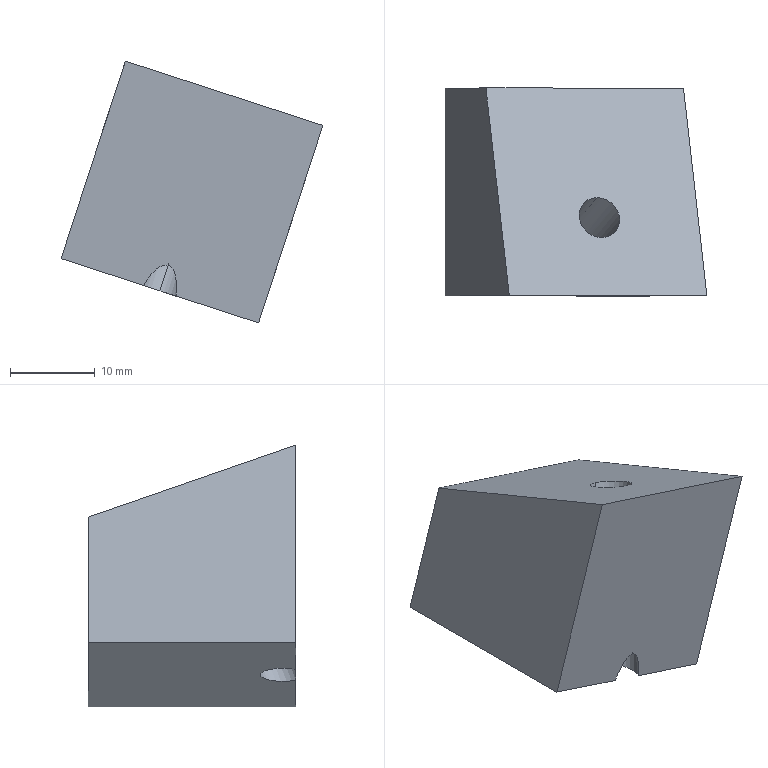Part | STEP file | 1 solid | 12 faces | box 30.872 x 24.5 x 30.872 mm | volume 11423 mm3 | plane 6 | cylinder 4 | cone 2 | commonest cylinder face diameters 4.165 x2 4.998 x2
STEP:
#1=CARTESIAN_POINT('',(0.,0.,0.));
#2=DIRECTION('',(0.,0.,1.));
#3=DIRECTION('',(1.,0.,0.));
#4=AXIS2_PLACEMENT_3D('',#1,#2,#3);
#5=CARTESIAN_POINT('',(844.273,-70.314,183.907));
#6=VERTEX_POINT('',#5);
#7=CARTESIAN_POINT('',(848.234,-70.314,182.62));
#8=VERTEX_POINT('',#7);
#9=CARTESIAN_POINT('',(846.254,-70.314,183.263));
#10=DIRECTION('',(0.,1.,0.));
#11=DIRECTION('',(-0.9511,0.,0.309));
#12=AXIS2_PLACEMENT_3D('',#9,#10,#11);
#13=CIRCLE('',#12,2.083);
#14=CARTESIAN_POINT('',(846.254,-70.314,183.263));
#15=DIRECTION('',(0.,1.,0.));
#16=DIRECTION('',(-0.9511,0.,0.309));
#17=AXIS2_PLACEMENT_3D('',#14,#15,#16);
#18=CONICAL_SURFACE('',#17,2.083,1.03);
#19=CARTESIAN_POINT('',(0.,0.));
#20=DIRECTION('',(1.,0.));
#21=VECTOR('',#20,1.);
#22=LINE('',#19,#21);
#23=(GEOMETRIC_REPRESENTATION_CONTEXT(2)PARAMETRIC_REPRESENTATION_CONTEXT()REPRESENTATION_CONTEXT('',''));
#24=DEFINITIONAL_REPRESENTATION('',(#22),#23);
#25=PCURVE('',#18,#24);
#26=CARTESIAN_POINT('',(846.254,-58.309,183.263));
#27=DIRECTION('',(0.,1.,0.));
#28=DIRECTION('',(-0.9511,0.,0.309));
#29=AXIS2_PLACEMENT_3D('',#26,#27,#28);
#30=CYLINDRICAL_SURFACE('',#29,2.083);
#31=CARTESIAN_POINT('',(0.,-12.005));
#32=DIRECTION('',(1.,0.));
#33=VECTOR('',#32,1.);
#34=LINE('',#31,#33);
#35=(GEOMETRIC_REPRESENTATION_CONTEXT(2)PARAMETRIC_REPRESENTATION_CONTEXT()REPRESENTATION_CONTEXT('',''));
#36=DEFINITIONAL_REPRESENTATION('',(#34),#35);
#37=PCURVE('',#30,#36);
#38=SURFACE_CURVE('',#13,(#25,#37),.PCURVE_S1.);
#39=EDGE_CURVE('',#6,#8,#38,.T.);
#40=ORIENTED_EDGE('',*,*,#39,.F.);
#41=CARTESIAN_POINT('',(846.254,-71.565,183.263));
#42=VERTEX_POINT('',#41);
#43=CARTESIAN_POINT('',(844.273,-70.314,183.907));
#44=DIRECTION('',(-0.8152,0.515,0.2649));
#45=VECTOR('',#44,1.);
#46=LINE('',#43,#45);
#47=CARTESIAN_POINT('',(0.,-1.251));
#48=CARTESIAN_POINT('',(0.,-1.232));
#49=CARTESIAN_POINT('',(0.,-1.194));
#50=CARTESIAN_POINT('',(0.,-1.138));
#51=CARTESIAN_POINT('',(0.,-1.081));
#52=CARTESIAN_POINT('',(0.,-1.024));
#53=CARTESIAN_POINT('',(0.,-0.9669));
#54=CARTESIAN_POINT('',(0.,-0.91));
#55=CARTESIAN_POINT('',(0.,-0.8532));
#56=CARTESIAN_POINT('',(0.,-0.7963));
#57=CARTESIAN_POINT('',(0.,-0.7394));
#58=CARTESIAN_POINT('',(0.,-0.6825));
#59=CARTESIAN_POINT('',(0.,-0.6256));
#60=CARTESIAN_POINT('',(0.,-0.5688));
#61=CARTESIAN_POINT('',(0.,-0.5119));
#62=CARTESIAN_POINT('',(0.,-0.455));
#63=CARTESIAN_POINT('',(0.,-0.3981));
#64=CARTESIAN_POINT('',(0.,-0.3413));
#65=CARTESIAN_POINT('',(0.,-0.2844));
#66=CARTESIAN_POINT('',(0.,-0.2275));
#67=CARTESIAN_POINT('',(0.,-0.1706));
#68=CARTESIAN_POINT('',(0.,-0.1138));
#69=CARTESIAN_POINT('',(0.,-0.05688));
#70=CARTESIAN_POINT('',(0.,-0.01896));
#71=CARTESIAN_POINT('',(0.,0.));
#72=B_SPLINE_CURVE_WITH_KNOTS('',3,(#47,#48,#49,#50,#51,#52,#53,#54,#55,#56,#57,#58,#59,#60,#61,#62,#63,#64,#65,#66,#67,#68,#69,#70,#71),.UNSPECIFIED.,.F.,.F.,(4,1,1,1,1,1,1,1,1,1,1,1,1,1,1,1,1,1,1,1,1,1,4),(-2.43,-2.319,-2.209,-2.098,-1.988,-1.877,-1.767,-1.656,-1.546,-1.436,-1.325,-1.215,-1.104,-0.9939,-0.8835,-0.773,-0.6626,-0.5522,-0.4417,-0.3313,-0.2209,-0.1104,0.),.UNSPECIFIED.);
#73=(GEOMETRIC_REPRESENTATION_CONTEXT(2)PARAMETRIC_REPRESENTATION_CONTEXT()REPRESENTATION_CONTEXT('',''));
#74=DEFINITIONAL_REPRESENTATION('',(#72),#73);
#75=PCURVE('',#18,#74);
#76=CARTESIAN_POINT('',(846.254,-70.314,183.263));
#77=DIRECTION('',(0.,1.,0.));
#78=DIRECTION('',(-0.9511,0.,0.309));
#79=AXIS2_PLACEMENT_3D('',#76,#77,#78);
#80=CONICAL_SURFACE('',#79,2.083,1.03);
#81=CARTESIAN_POINT('',(6.283,-1.251));
#82=CARTESIAN_POINT('',(6.283,-1.232));
#83=CARTESIAN_POINT('',(6.283,-1.194));
#84=CARTESIAN_POINT('',(6.283,-1.138));
#85=CARTESIAN_POINT('',(6.283,-1.081));
#86=CARTESIAN_POINT('',(6.283,-1.024));
#87=CARTESIAN_POINT('',(6.283,-0.9669));
#88=CARTESIAN_POINT('',(6.283,-0.91));
#89=CARTESIAN_POINT('',(6.283,-0.8532));
#90=CARTESIAN_POINT('',(6.283,-0.7963));
#91=CARTESIAN_POINT('',(6.283,-0.7394));
#92=CARTESIAN_POINT('',(6.283,-0.6825));
#93=CARTESIAN_POINT('',(6.283,-0.6256));
#94=CARTESIAN_POINT('',(6.283,-0.5688));
#95=CARTESIAN_POINT('',(6.283,-0.5119));
#96=CARTESIAN_POINT('',(6.283,-0.455));
#97=CARTESIAN_POINT('',(6.283,-0.3981));
#98=CARTESIAN_POINT('',(6.283,-0.3413));
#99=CARTESIAN_POINT('',(6.283,-0.2844));
#100=CARTESIAN_POINT('',(6.283,-0.2275));
#101=CARTESIAN_POINT('',(6.283,-0.1706));
#102=CARTESIAN_POINT('',(6.283,-0.1138));
#103=CARTESIAN_POINT('',(6.283,-0.05688));
#104=CARTESIAN_POINT('',(6.283,-0.01896));
#105=CARTESIAN_POINT('',(6.283,0.));
#106=B_SPLINE_CURVE_WITH_KNOTS('',3,(#81,#82,#83,#84,#85,#86,#87,#88,#89,#90,#91,#92,#93,#94,#95,#96,#97,#98,#99,#100,#101,#102,#103,#104,#105),.UNSPECIFIED.,.F.,.F.,(4,1,1,1,1,1,1,1,1,1,1,1,1,1,1,1,1,1,1,1,1,1,4),(-2.43,-2.319,-2.209,-2.098,-1.988,-1.877,-1.767,-1.656,-1.546,-1.436,-1.325,-1.215,-1.104,-0.9939,-0.8835,-0.773,-0.6626,-0.5522,-0.4417,-0.3313,-0.2209,-0.1104,0.),.UNSPECIFIED.);
#107=(GEOMETRIC_REPRESENTATION_CONTEXT(2)PARAMETRIC_REPRESENTATION_CONTEXT()REPRESENTATION_CONTEXT('',''));
#108=DEFINITIONAL_REPRESENTATION('',(#106),#107);
#109=PCURVE('',#80,#108);
#110=SURFACE_CURVE('',#46,(#75,#109),.PCURVE_S1.);
#111=EDGE_CURVE('',#42,#6,#110,.T.);
#112=ORIENTED_EDGE('',*,*,#111,.F.);
#113=CARTESIAN_POINT('',(848.234,-70.314,182.62));
#114=DIRECTION('',(0.8152,0.515,-0.2649));
#115=VECTOR('',#114,1.);
#116=LINE('',#113,#115);
#117=CARTESIAN_POINT('',(3.142,-1.251));
#118=CARTESIAN_POINT('',(3.142,-1.232));
#119=CARTESIAN_POINT('',(3.142,-1.194));
#120=CARTESIAN_POINT('',(3.142,-1.138));
#121=CARTESIAN_POINT('',(3.142,-1.081));
#122=CARTESIAN_POINT('',(3.142,-1.024));
#123=CARTESIAN_POINT('',(3.142,-0.9669));
#124=CARTESIAN_POINT('',(3.142,-0.91));
#125=CARTESIAN_POINT('',(3.142,-0.8532));
#126=CARTESIAN_POINT('',(3.142,-0.7963));
#127=CARTESIAN_POINT('',(3.142,-0.7394));
#128=CARTESIAN_POINT('',(3.142,-0.6825));
#129=CARTESIAN_POINT('',(3.142,-0.6256));
#130=CARTESIAN_POINT('',(3.142,-0.5688));
#131=CARTESIAN_POINT('',(3.142,-0.5119));
#132=CARTESIAN_POINT('',(3.142,-0.455));
#133=CARTESIAN_POINT('',(3.142,-0.3981));
#134=CARTESIAN_POINT('',(3.142,-0.3413));
#135=CARTESIAN_POINT('',(3.142,-0.2844));
#136=CARTESIAN_POINT('',(3.142,-0.2275));
#137=CARTESIAN_POINT('',(3.142,-0.1706));
#138=CARTESIAN_POINT('',(3.142,-0.1138));
#139=CARTESIAN_POINT('',(3.142,-0.05688));
#140=CARTESIAN_POINT('',(3.142,-0.01896));
#141=CARTESIAN_POINT('',(3.142,0.));
#142=B_SPLINE_CURVE_WITH_KNOTS('',3,(#117,#118,#119,#120,#121,#122,#123,#124,#125,#126,#127,#128,#129,#130,#131,#132,#133,#134,#135,#136,#137,#138,#139,#140,#141),.UNSPECIFIED.,.F.,.F.,(4,1,1,1,1,1,1,1,1,1,1,1,1,1,1,1,1,1,1,1,1,1,4),(-2.43,-2.319,-2.209,-2.098,-1.988,-1.877,-1.767,-1.656,-1.546,-1.436,-1.325,-1.215,-1.104,-0.9939,-0.8835,-0.773,-0.6626,-0.5522,-0.4417,-0.3313,-0.2209,-0.1104,0.),.UNSPECIFIED.);
#143=(GEOMETRIC_REPRESENTATION_CONTEXT(2)PARAMETRIC_REPRESENTATION_CONTEXT()REPRESENTATION_CONTEXT('',''));
#144=DEFINITIONAL_REPRESENTATION('',(#142),#143);
#145=PCURVE('',#18,#144);
#146=CARTESIAN_POINT('',(3.142,-1.251));
#147=CARTESIAN_POINT('',(3.142,-1.232));
#148=CARTESIAN_POINT('',(3.142,-1.194));
#149=CARTESIAN_POINT('',(3.142,-1.138));
#150=CARTESIAN_POINT('',(3.142,-1.081));
#151=CARTESIAN_POINT('',(3.142,-1.024));
#152=CARTESIAN_POINT('',(3.142,-0.9669));
#153=CARTESIAN_POINT('',(3.142,-0.91));
#154=CARTESIAN_POINT('',(3.142,-0.8532));
#155=CARTESIAN_POINT('',(3.142,-0.7963));
#156=CARTESIAN_POINT('',(3.142,-0.7394));
#157=CARTESIAN_POINT('',(3.142,-0.6825));
#158=CARTESIAN_POINT('',(3.142,-0.6256));
#159=CARTESIAN_POINT('',(3.142,-0.5688));
#160=CARTESIAN_POINT('',(3.142,-0.5119));
#161=CARTESIAN_POINT('',(3.142,-0.455));
#162=CARTESIAN_POINT('',(3.142,-0.3981));
#163=CARTESIAN_POINT('',(3.142,-0.3413));
#164=CARTESIAN_POINT('',(3.142,-0.2844));
#165=CARTESIAN_POINT('',(3.142,-0.2275));
#166=CARTESIAN_POINT('',(3.142,-0.1706));
#167=CARTESIAN_POINT('',(3.142,-0.1138));
#168=CARTESIAN_POINT('',(3.142,-0.05688));
#169=CARTESIAN_POINT('',(3.142,-0.01896));
#170=CARTESIAN_POINT('',(3.142,0.));
#171=B_SPLINE_CURVE_WITH_KNOTS('',3,(#146,#147,#148,#149,#150,#151,#152,#153,#154,#155,#156,#157,#158,#159,#160,#161,#162,#163,#164,#165,#166,#167,#168,#169,#170),.UNSPECIFIED.,.F.,.F.,(4,1,1,1,1,1,1,1,1,1,1,1,1,1,1,1,1,1,1,1,1,1,4),(-2.43,-2.319,-2.209,-2.098,-1.988,-1.877,-1.767,-1.656,-1.546,-1.436,-1.325,-1.215,-1.104,-0.9939,-0.8835,-0.773,-0.6626,-0.5522,-0.4417,-0.3313,-0.2209,-0.1104,0.),.UNSPECIFIED.);
#172=(GEOMETRIC_REPRESENTATION_CONTEXT(2)PARAMETRIC_REPRESENTATION_CONTEXT()REPRESENTATION_CONTEXT('',''));
#173=DEFINITIONAL_REPRESENTATION('',(#171),#172);
#174=PCURVE('',#80,#173);
#175=SURFACE_CURVE('',#116,(#145,#174),.PCURVE_S1.);
#176=EDGE_CURVE('',#42,#8,#175,.T.);
#177=ORIENTED_EDGE('',*,*,#176,.T.);
#178=EDGE_LOOP('',(#40,#112,#177));
#179=FACE_BOUND('',#178,.F.);
#180=ADVANCED_FACE('',(#179),#18,.F.);
#181=CARTESIAN_POINT('',(844.273,-58.309,183.907));
#182=VERTEX_POINT('',#181);
#183=CARTESIAN_POINT('',(848.234,-58.309,182.62));
#184=VERTEX_POINT('',#183);
#185=CARTESIAN_POINT('',(846.254,-58.309,183.263));
#186=DIRECTION('',(0.,1.,0.));
#187=DIRECTION('',(-0.9511,0.,0.309));
#188=AXIS2_PLACEMENT_3D('',#185,#186,#187);
#189=CIRCLE('',#188,2.083);
#190=CARTESIAN_POINT('',(0.,0.));
#191=DIRECTION('',(1.,0.));
#192=VECTOR('',#191,1.);
#193=LINE('',#190,#192);
#194=(GEOMETRIC_REPRESENTATION_CONTEXT(2)PARAMETRIC_REPRESENTATION_CONTEXT()REPRESENTATION_CONTEXT('',''));
#195=DEFINITIONAL_REPRESENTATION('',(#193),#194);
#196=PCURVE('',#30,#195);
#197=CARTESIAN_POINT('',(837.147,-58.309,194.878));
#198=DIRECTION('',(0.,-1.,0.));
#199=DIRECTION('',(0.9511,0.,-0.309));
#200=AXIS2_PLACEMENT_3D('',#197,#198,#199);
#201=PLANE('',#200);
#202=CARTESIAN_POINT('',(10.168,-8.233));
#203=CARTESIAN_POINT('',(10.168,-4.626));
#204=CARTESIAN_POINT('',(13.291,-6.429));
#205=CARTESIAN_POINT('',(16.415,-8.233));
#206=CARTESIAN_POINT('',(13.291,-10.036));
#207=CARTESIAN_POINT('',(10.168,-11.84));
#208=CARTESIAN_POINT('',(10.168,-8.233));
#209=(BOUNDED_CURVE()B_SPLINE_CURVE(2,(#202,#203,#204,#205,#206,#207,#208),.UNSPECIFIED.,.T.,.F.)B_SPLINE_CURVE_WITH_KNOTS((1,2,2,2,2,1),(-2.094,0.,2.094,4.189,6.283,8.378),.UNSPECIFIED.)CURVE()GEOMETRIC_REPRESENTATION_ITEM()RATIONAL_B_SPLINE_CURVE((1.,0.5,1.,0.5,1.,0.5,1.))REPRESENTATION_ITEM(''));
#210=(GEOMETRIC_REPRESENTATION_CONTEXT(2)PARAMETRIC_REPRESENTATION_CONTEXT()REPRESENTATION_CONTEXT('',''));
#211=DEFINITIONAL_REPRESENTATION('',(#209),#210);
#212=PCURVE('',#201,#211);
#213=SURFACE_CURVE('',#189,(#196,#212),.PCURVE_S1.);
#214=EDGE_CURVE('',#182,#184,#213,.T.);
#215=ORIENTED_EDGE('',*,*,#214,.F.);
#216=CARTESIAN_POINT('',(844.273,-58.309,183.907));
#217=DIRECTION('',(0.,1.,0.));
#218=VECTOR('',#217,1.);
#219=LINE('',#216,#218);
#220=CARTESIAN_POINT('',(0.,0.));
#221=DIRECTION('',(0.,1.));
#222=VECTOR('',#221,1.);
#223=LINE('',#220,#222);
#224=(GEOMETRIC_REPRESENTATION_CONTEXT(2)PARAMETRIC_REPRESENTATION_CONTEXT()REPRESENTATION_CONTEXT('',''));
#225=DEFINITIONAL_REPRESENTATION('',(#223),#224);
#226=PCURVE('',#30,#225);
#227=CARTESIAN_POINT('',(846.254,-58.309,183.263));
#228=DIRECTION('',(0.,1.,0.));
#229=DIRECTION('',(-0.9511,0.,0.309));
#230=AXIS2_PLACEMENT_3D('',#227,#228,#229);
#231=CYLINDRICAL_SURFACE('',#230,2.083);
#232=CARTESIAN_POINT('',(6.283,0.));
#233=DIRECTION('',(0.,1.));
#234=VECTOR('',#233,1.);
#235=LINE('',#232,#234);
#236=(GEOMETRIC_REPRESENTATION_CONTEXT(2)PARAMETRIC_REPRESENTATION_CONTEXT()REPRESENTATION_CONTEXT('',''));
#237=DEFINITIONAL_REPRESENTATION('',(#235),#236);
#238=PCURVE('',#231,#237);
#239=SURFACE_CURVE('',#219,(#226,#238),.PCURVE_S1.);
#240=EDGE_CURVE('',#6,#182,#239,.T.);
#241=ORIENTED_EDGE('',*,*,#240,.F.);
#242=ORIENTED_EDGE('',*,*,#39,.T.);
#243=CARTESIAN_POINT('',(848.234,-58.309,182.62));
#244=DIRECTION('',(0.,1.,0.));
#245=VECTOR('',#244,1.);
#246=LINE('',#243,#245);
#247=CARTESIAN_POINT('',(3.142,0.));
#248=DIRECTION('',(0.,1.));
#249=VECTOR('',#248,1.);
#250=LINE('',#247,#249);
#251=(GEOMETRIC_REPRESENTATION_CONTEXT(2)PARAMETRIC_REPRESENTATION_CONTEXT()REPRESENTATION_CONTEXT('',''));
#252=DEFINITIONAL_REPRESENTATION('',(#250),#251);
#253=PCURVE('',#30,#252);
#254=CARTESIAN_POINT('',(3.142,0.));
#255=DIRECTION('',(0.,1.));
#256=VECTOR('',#255,1.);
#257=LINE('',#254,#256);
#258=(GEOMETRIC_REPRESENTATION_CONTEXT(2)PARAMETRIC_REPRESENTATION_CONTEXT()REPRESENTATION_CONTEXT('',''));
#259=DEFINITIONAL_REPRESENTATION('',(#257),#258);
#260=PCURVE('',#231,#259);
#261=SURFACE_CURVE('',#246,(#253,#260),.PCURVE_S1.);
#262=EDGE_CURVE('',#8,#184,#261,.T.);
#263=ORIENTED_EDGE('',*,*,#262,.T.);
#264=EDGE_LOOP('',(#215,#241,#242,#263));
#265=FACE_BOUND('',#264,.F.);
#266=ADVANCED_FACE('',(#265),#30,.F.);
#267=CARTESIAN_POINT('',(855.633,-82.809,172.487));
#268=VERTEX_POINT('',#267);
#269=CARTESIAN_POINT('',(845.938,-82.809,175.638));
#270=VERTEX_POINT('',#269);
#271=CARTESIAN_POINT('',(832.332,-82.809,180.058));
#272=DIRECTION('',(-0.9511,0.,0.309));
#273=VECTOR('',#272,1.);
#274=LINE('',#271,#273);
#275=CARTESIAN_POINT('',(832.332,-58.309,180.058));
#276=DIRECTION('',(0.309,0.,0.9511));
#277=DIRECTION('',(0.,1.,0.));
#278=AXIS2_PLACEMENT_3D('',#275,#276,#277);
#279=PLANE('',#278);
#280=CARTESIAN_POINT('',(-24.5,0.));
#281=DIRECTION('',(0.,1.));
#282=VECTOR('',#281,1.);
#283=LINE('',#280,#282);
#284=(GEOMETRIC_REPRESENTATION_CONTEXT(2)PARAMETRIC_REPRESENTATION_CONTEXT()REPRESENTATION_CONTEXT('',''));
#285=DEFINITIONAL_REPRESENTATION('',(#283),#284);
#286=PCURVE('',#279,#285);
#287=CARTESIAN_POINT('',(832.332,-82.809,180.058));
#288=DIRECTION('',(0.,1.,0.));
#289=DIRECTION('',(0.309,0.,0.9511));
#290=AXIS2_PLACEMENT_3D('',#287,#288,#289);
#291=PLANE('',#290);
#292=CARTESIAN_POINT('',(0.,0.));
#293=DIRECTION('',(0.,-1.));
#294=VECTOR('',#293,1.);
#295=LINE('',#292,#294);
#296=(GEOMETRIC_REPRESENTATION_CONTEXT(2)PARAMETRIC_REPRESENTATION_CONTEXT()REPRESENTATION_CONTEXT('',''));
#297=DEFINITIONAL_REPRESENTATION('',(#295),#296);
#298=PCURVE('',#291,#297);
#299=SURFACE_CURVE('',#274,(#286,#298),.PCURVE_S1.);
#300=EDGE_CURVE('',#268,#270,#299,.T.);
#301=ORIENTED_EDGE('',*,*,#300,.T.);
#302=CARTESIAN_POINT('',(843.983,-78.638,176.273));
#303=VERTEX_POINT('',#302);
#304=CARTESIAN_POINT('',(845.938,-82.809,175.638));
#305=CARTESIAN_POINT('',(847.178,-80.8,175.235));
#306=CARTESIAN_POINT('',(846.165,-78.638,175.564));
#307=CARTESIAN_POINT('',(843.983,-78.638,176.273));
#308=(BOUNDED_CURVE()B_SPLINE_CURVE(3,(#304,#305,#306,#307),.UNSPECIFIED.,.F.,.F.)B_SPLINE_CURVE_WITH_KNOTS((4,4),(4.108,6.283),.PIECEWISE_BEZIER_KNOTS.)CURVE()GEOMETRIC_REPRESENTATION_ITEM()RATIONAL_B_SPLINE_CURVE((1.,0.643,0.643,1.))REPRESENTATION_ITEM(''));
#309=CARTESIAN_POINT('',(-24.5,-14.306));
#310=CARTESIAN_POINT('',(-22.491,-15.61));
#311=CARTESIAN_POINT('',(-20.329,-14.544));
#312=CARTESIAN_POINT('',(-20.329,-12.25));
#313=(BOUNDED_CURVE()B_SPLINE_CURVE(3,(#309,#310,#311,#312),.UNSPECIFIED.,.F.,.F.)B_SPLINE_CURVE_WITH_KNOTS((4,4),(4.108,6.283),.PIECEWISE_BEZIER_KNOTS.)CURVE()GEOMETRIC_REPRESENTATION_ITEM()RATIONAL_B_SPLINE_CURVE((1.,0.643,0.643,1.))REPRESENTATION_ITEM(''));
#314=(GEOMETRIC_REPRESENTATION_CONTEXT(2)PARAMETRIC_REPRESENTATION_CONTEXT()REPRESENTATION_CONTEXT('',''));
#315=DEFINITIONAL_REPRESENTATION('',(#313),#314);
#316=PCURVE('',#279,#315);
#317=CARTESIAN_POINT('',(850.518,-73.6,196.386));
#318=DIRECTION('',(0.2904,0.342,0.8937));
#319=DIRECTION('',(-0.1057,0.9397,-0.3253));
#320=AXIS2_PLACEMENT_3D('',#317,#318,#319);
#321=CYLINDRICAL_SURFACE('',#320,2.499);
#322=CARTESIAN_POINT('',(4.108,-23.022));
#323=CARTESIAN_POINT('',(4.135,-23.002));
#324=CARTESIAN_POINT('',(4.19,-22.96));
#325=CARTESIAN_POINT('',(4.276,-22.89));
#326=CARTESIAN_POINT('',(4.366,-22.814));
#327=CARTESIAN_POINT('',(4.46,-22.733));
#328=CARTESIAN_POINT('',(4.558,-22.646));
#329=CARTESIAN_POINT('',(4.659,-22.554));
#330=CARTESIAN_POINT('',(4.762,-22.46));
#331=CARTESIAN_POINT('',(4.868,-22.364));
#332=CARTESIAN_POINT('',(4.976,-22.268));
#333=CARTESIAN_POINT('',(5.086,-22.173));
#334=CARTESIAN_POINT('',(5.195,-22.082));
#335=CARTESIAN_POINT('',(5.305,-21.996));
#336=CARTESIAN_POINT('',(5.415,-21.917));
#337=CARTESIAN_POINT('',(5.523,-21.845));
#338=CARTESIAN_POINT('',(5.629,-21.782));
#339=CARTESIAN_POINT('',(5.732,-21.729));
#340=CARTESIAN_POINT('',(5.833,-21.685));
#341=CARTESIAN_POINT('',(5.931,-21.65));
#342=CARTESIAN_POINT('',(6.025,-21.625));
#343=CARTESIAN_POINT('',(6.115,-21.608));
#344=CARTESIAN_POINT('',(6.201,-21.598));
#345=CARTESIAN_POINT('',(6.256,-21.596));
#346=CARTESIAN_POINT('',(6.283,-21.596));
#347=B_SPLINE_CURVE_WITH_KNOTS('',3,(#322,#323,#324,#325,#326,#327,#328,#329,#330,#331,#332,#333,#334,#335,#336,#337,#338,#339,#340,#341,#342,#343,#344,#345,#346),.UNSPECIFIED.,.F.,.F.,(4,1,1,1,1,1,1,1,1,1,1,1,1,1,1,1,1,1,1,1,1,1,4),(4.108,4.207,4.306,4.404,4.503,4.602,4.701,4.8,4.899,4.998,5.097,5.195,5.294,5.393,5.492,5.591,5.69,5.789,5.888,5.987,6.085,6.184,6.283),.QUASI_UNIFORM_KNOTS.);
#348=(GEOMETRIC_REPRESENTATION_CONTEXT(2)PARAMETRIC_REPRESENTATION_CONTEXT()REPRESENTATION_CONTEXT('',''));
#349=DEFINITIONAL_REPRESENTATION('',(#347),#348);
#350=PCURVE('',#321,#349);
#351=SURFACE_CURVE('',#308,(#316,#350),.PCURVE_S1.);
#352=EDGE_CURVE('',#270,#303,#351,.T.);
#353=ORIENTED_EDGE('',*,*,#352,.T.);
#354=CARTESIAN_POINT('',(842.027,-82.809,176.908));
#355=VERTEX_POINT('',#354);
#356=CARTESIAN_POINT('',(843.983,-78.638,176.273));
#357=CARTESIAN_POINT('',(841.8,-78.638,176.982));
#358=CARTESIAN_POINT('',(840.787,-80.8,177.311));
#359=CARTESIAN_POINT('',(842.027,-82.809,176.908));
#360=(BOUNDED_CURVE()B_SPLINE_CURVE(3,(#356,#357,#358,#359),.UNSPECIFIED.,.F.,.F.)B_SPLINE_CURVE_WITH_KNOTS((4,4),(0.,2.175),.PIECEWISE_BEZIER_KNOTS.)CURVE()GEOMETRIC_REPRESENTATION_ITEM()RATIONAL_B_SPLINE_CURVE((1.,0.643,0.643,1.))REPRESENTATION_ITEM(''));
#361=CARTESIAN_POINT('',(-20.329,-12.25));
#362=CARTESIAN_POINT('',(-20.329,-9.956));
#363=CARTESIAN_POINT('',(-22.491,-8.89));
#364=CARTESIAN_POINT('',(-24.5,-10.194));
#365=(BOUNDED_CURVE()B_SPLINE_CURVE(3,(#361,#362,#363,#364),.UNSPECIFIED.,.F.,.F.)B_SPLINE_CURVE_WITH_KNOTS((4,4),(0.,2.175),.PIECEWISE_BEZIER_KNOTS.)CURVE()GEOMETRIC_REPRESENTATION_ITEM()RATIONAL_B_SPLINE_CURVE((1.,0.643,0.643,1.))REPRESENTATION_ITEM(''));
#366=(GEOMETRIC_REPRESENTATION_CONTEXT(2)PARAMETRIC_REPRESENTATION_CONTEXT()REPRESENTATION_CONTEXT('',''));
#367=DEFINITIONAL_REPRESENTATION('',(#365),#366);
#368=PCURVE('',#279,#367);
#369=CARTESIAN_POINT('',(850.518,-73.6,196.386));
#370=DIRECTION('',(0.2904,0.342,0.8937));
#371=DIRECTION('',(-0.1057,0.9397,-0.3253));
#372=AXIS2_PLACEMENT_3D('',#369,#370,#371);
#373=CYLINDRICAL_SURFACE('',#372,2.499);
#374=CARTESIAN_POINT('',(0.,-21.596));
#375=CARTESIAN_POINT('',(0.02683,-21.596));
#376=CARTESIAN_POINT('',(0.08182,-21.598));
#377=CARTESIAN_POINT('',(0.1682,-21.608));
#378=CARTESIAN_POINT('',(0.2585,-21.625));
#379=CARTESIAN_POINT('',(0.3525,-21.65));
#380=CARTESIAN_POINT('',(0.45,-21.685));
#381=CARTESIAN_POINT('',(0.5508,-21.729));
#382=CARTESIAN_POINT('',(0.6544,-21.782));
#383=CARTESIAN_POINT('',(0.7605,-21.845));
#384=CARTESIAN_POINT('',(0.8685,-21.917));
#385=CARTESIAN_POINT('',(0.9778,-21.996));
#386=CARTESIAN_POINT('',(1.088,-22.082));
#387=CARTESIAN_POINT('',(1.198,-22.173));
#388=CARTESIAN_POINT('',(1.307,-22.268));
#389=CARTESIAN_POINT('',(1.415,-22.364));
#390=CARTESIAN_POINT('',(1.521,-22.46));
#391=CARTESIAN_POINT('',(1.625,-22.554));
#392=CARTESIAN_POINT('',(1.725,-22.646));
#393=CARTESIAN_POINT('',(1.823,-22.733));
#394=CARTESIAN_POINT('',(1.917,-22.814));
#395=CARTESIAN_POINT('',(2.007,-22.89));
#396=CARTESIAN_POINT('',(2.094,-22.96));
#397=CARTESIAN_POINT('',(2.149,-23.002));
#398=CARTESIAN_POINT('',(2.175,-23.022));
#399=B_SPLINE_CURVE_WITH_KNOTS('',3,(#374,#375,#376,#377,#378,#379,#380,#381,#382,#383,#384,#385,#386,#387,#388,#389,#390,#391,#392,#393,#394,#395,#396,#397,#398),.UNSPECIFIED.,.F.,.F.,(4,1,1,1,1,1,1,1,1,1,1,1,1,1,1,1,1,1,1,1,1,1,4),(0.,0.09888,0.1978,0.2966,0.3955,0.4944,0.5933,0.6922,0.7911,0.8899,0.9888,1.088,1.187,1.285,1.384,1.483,1.582,1.681,1.78,1.879,1.978,2.077,2.175),.QUASI_UNIFORM_KNOTS.);
#400=(GEOMETRIC_REPRESENTATION_CONTEXT(2)PARAMETRIC_REPRESENTATION_CONTEXT()REPRESENTATION_CONTEXT('',''));
#401=DEFINITIONAL_REPRESENTATION('',(#399),#400);
#402=PCURVE('',#373,#401);
#403=SURFACE_CURVE('',#360,(#368,#402),.PCURVE_S1.);
#404=EDGE_CURVE('',#303,#355,#403,.T.);
#405=ORIENTED_EDGE('',*,*,#404,.T.);
#406=CARTESIAN_POINT('',(832.332,-82.809,180.058));
#407=VERTEX_POINT('',#406);
#408=CARTESIAN_POINT('',(832.332,-82.809,180.058));
#409=DIRECTION('',(-0.9511,0.,0.309));
#410=VECTOR('',#409,1.);
#411=LINE('',#408,#410);
#412=CARTESIAN_POINT('',(-24.5,0.));
#413=DIRECTION('',(0.,1.));
#414=VECTOR('',#413,1.);
#415=LINE('',#412,#414);
#416=(GEOMETRIC_REPRESENTATION_CONTEXT(2)PARAMETRIC_REPRESENTATION_CONTEXT()REPRESENTATION_CONTEXT('',''));
#417=DEFINITIONAL_REPRESENTATION('',(#415),#416);
#418=PCURVE('',#279,#417);
#419=CARTESIAN_POINT('',(0.,0.));
#420=DIRECTION('',(0.,-1.));
#421=VECTOR('',#420,1.);
#422=LINE('',#419,#421);
#423=(GEOMETRIC_REPRESENTATION_CONTEXT(2)PARAMETRIC_REPRESENTATION_CONTEXT()REPRESENTATION_CONTEXT('',''));
#424=DEFINITIONAL_REPRESENTATION('',(#422),#423);
#425=PCURVE('',#291,#424);
#426=SURFACE_CURVE('',#411,(#418,#425),.PCURVE_S1.);
#427=EDGE_CURVE('',#355,#407,#426,.T.);
#428=ORIENTED_EDGE('',*,*,#427,.T.);
#429=CARTESIAN_POINT('',(832.332,-58.309,180.058));
#430=VERTEX_POINT('',#429);
#431=CARTESIAN_POINT('',(832.332,-82.809,180.058));
#432=DIRECTION('',(0.,-1.,0.));
#433=VECTOR('',#432,1.);
#434=LINE('',#431,#433);
#435=CARTESIAN_POINT('',(-24.5,0.));
#436=DIRECTION('',(-1.,0.));
#437=VECTOR('',#436,1.);
#438=LINE('',#435,#437);
#439=(GEOMETRIC_REPRESENTATION_CONTEXT(2)PARAMETRIC_REPRESENTATION_CONTEXT()REPRESENTATION_CONTEXT('',''));
#440=DEFINITIONAL_REPRESENTATION('',(#438),#439);
#441=PCURVE('',#279,#440);
#442=CARTESIAN_POINT('',(832.332,-82.809,180.058));
#443=DIRECTION('',(-0.9511,0.,0.309));
#444=DIRECTION('',(0.309,0.,0.9511));
#445=AXIS2_PLACEMENT_3D('',#442,#443,#444);
#446=PLANE('',#445);
#447=CARTESIAN_POINT('',(0.,0.));
#448=DIRECTION('',(0.,-1.));
#449=VECTOR('',#448,1.);
#450=LINE('',#447,#449);
#451=(GEOMETRIC_REPRESENTATION_CONTEXT(2)PARAMETRIC_REPRESENTATION_CONTEXT()REPRESENTATION_CONTEXT('',''));
#452=DEFINITIONAL_REPRESENTATION('',(#450),#451);
#453=PCURVE('',#446,#452);
#454=SURFACE_CURVE('',#434,(#441,#453),.PCURVE_S1.);
#455=EDGE_CURVE('',#430,#407,#454,.T.);
#456=ORIENTED_EDGE('',*,*,#455,.F.);
#457=CARTESIAN_POINT('',(855.633,-58.309,172.487));
#458=VERTEX_POINT('',#457);
#459=CARTESIAN_POINT('',(832.332,-58.309,180.058));
#460=DIRECTION('',(0.9511,0.,-0.309));
#461=VECTOR('',#460,1.);
#462=LINE('',#459,#461);
#463=CARTESIAN_POINT('',(0.,0.));
#464=DIRECTION('',(0.,-1.));
#465=VECTOR('',#464,1.);
#466=LINE('',#463,#465);
#467=(GEOMETRIC_REPRESENTATION_CONTEXT(2)PARAMETRIC_REPRESENTATION_CONTEXT()REPRESENTATION_CONTEXT('',''));
#468=DEFINITIONAL_REPRESENTATION('',(#466),#467);
#469=PCURVE('',#279,#468);
#470=CARTESIAN_POINT('',(0.,-15.583));
#471=DIRECTION('',(1.,0.));
#472=VECTOR('',#471,1.);
#473=LINE('',#470,#472);
#474=(GEOMETRIC_REPRESENTATION_CONTEXT(2)PARAMETRIC_REPRESENTATION_CONTEXT()REPRESENTATION_CONTEXT('',''));
#475=DEFINITIONAL_REPRESENTATION('',(#473),#474);
#476=PCURVE('',#201,#475);
#477=SURFACE_CURVE('',#462,(#469,#476),.PCURVE_S1.);
#478=EDGE_CURVE('',#430,#458,#477,.T.);
#479=ORIENTED_EDGE('',*,*,#478,.T.);
#480=CARTESIAN_POINT('',(855.633,-82.809,172.487));
#481=DIRECTION('',(0.,-1.,0.));
#482=VECTOR('',#481,1.);
#483=LINE('',#480,#482);
#484=CARTESIAN_POINT('',(-24.5,-24.5));
#485=DIRECTION('',(-1.,0.));
#486=VECTOR('',#485,1.);
#487=LINE('',#484,#486);
#488=(GEOMETRIC_REPRESENTATION_CONTEXT(2)PARAMETRIC_REPRESENTATION_CONTEXT()REPRESENTATION_CONTEXT('',''));
#489=DEFINITIONAL_REPRESENTATION('',(#487),#488);
#490=PCURVE('',#279,#489);
#491=CARTESIAN_POINT('',(855.633,-82.809,172.487));
#492=DIRECTION('',(-0.9511,0.,0.309));
#493=DIRECTION('',(0.309,0.,0.9511));
#494=AXIS2_PLACEMENT_3D('',#491,#492,#493);
#495=PLANE('',#494);
#496=CARTESIAN_POINT('',(0.,0.));
#497=DIRECTION('',(0.,-1.));
#498=VECTOR('',#497,1.);
#499=LINE('',#496,#498);
#500=(GEOMETRIC_REPRESENTATION_CONTEXT(2)PARAMETRIC_REPRESENTATION_CONTEXT()REPRESENTATION_CONTEXT('',''));
#501=DEFINITIONAL_REPRESENTATION('',(#499),#500);
#502=PCURVE('',#495,#501);
#503=SURFACE_CURVE('',#483,(#490,#502),.PCURVE_S1.);
#504=EDGE_CURVE('',#458,#268,#503,.T.);
#505=ORIENTED_EDGE('',*,*,#504,.T.);
#506=EDGE_LOOP('',(#301,#353,#405,#428,#456,#479,#505));
#507=FACE_BOUND('',#506,.T.);
#508=ADVANCED_FACE('',(#507),#279,.F.);
#509=CARTESIAN_POINT('',(850.254,-71.252,195.573));
#510=VERTEX_POINT('',#509);
#511=CARTESIAN_POINT('',(850.782,-75.948,197.199));
#512=VERTEX_POINT('',#511);
#513=CARTESIAN_POINT('',(850.518,-73.6,196.386));
#514=DIRECTION('',(0.2904,0.342,0.8937));
#515=DIRECTION('',(-0.1057,0.9397,-0.3253));
#516=AXIS2_PLACEMENT_3D('',#513,#514,#515);
#517=CIRCLE('',#516,2.499);
#518=CARTESIAN_POINT('',(0.,0.));
#519=DIRECTION('',(1.,0.));
#520=VECTOR('',#519,1.);
#521=LINE('',#518,#520);
#522=(GEOMETRIC_REPRESENTATION_CONTEXT(2)PARAMETRIC_REPRESENTATION_CONTEXT()REPRESENTATION_CONTEXT('',''));
#523=DEFINITIONAL_REPRESENTATION('',(#521),#522);
#524=PCURVE('',#373,#523);
#525=CARTESIAN_POINT('',(839.903,-82.809,203.359));
#526=DIRECTION('',(-0.2904,-0.342,-0.8937));
#527=DIRECTION('',(-0.1057,0.9397,-0.3253));
#528=AXIS2_PLACEMENT_3D('',#525,#526,#527);
#529=PLANE('',#528);
#530=CARTESIAN_POINT('',(12.299,12.25));
#531=CARTESIAN_POINT('',(12.299,7.922));
#532=CARTESIAN_POINT('',(8.55,10.086));
#533=CARTESIAN_POINT('',(4.802,12.25));
#534=CARTESIAN_POINT('',(8.55,14.414));
#535=CARTESIAN_POINT('',(12.299,16.578));
#536=CARTESIAN_POINT('',(12.299,12.25));
#537=(BOUNDED_CURVE()B_SPLINE_CURVE(2,(#530,#531,#532,#533,#534,#535,#536),.UNSPECIFIED.,.T.,.F.)B_SPLINE_CURVE_WITH_KNOTS((1,2,2,2,2,1),(-2.094,0.,2.094,4.189,6.283,8.378),.UNSPECIFIED.)CURVE()GEOMETRIC_REPRESENTATION_ITEM()RATIONAL_B_SPLINE_CURVE((1.,0.5,1.,0.5,1.,0.5,1.))REPRESENTATION_ITEM(''));
#538=(GEOMETRIC_REPRESENTATION_CONTEXT(2)PARAMETRIC_REPRESENTATION_CONTEXT()REPRESENTATION_CONTEXT('',''));
#539=DEFINITIONAL_REPRESENTATION('',(#537),#538);
#540=PCURVE('',#529,#539);
#541=SURFACE_CURVE('',#517,(#524,#540),.PCURVE_S1.);
#542=EDGE_CURVE('',#510,#512,#541,.T.);
#543=ORIENTED_EDGE('',*,*,#542,.F.);
#544=CARTESIAN_POINT('',(850.254,-71.252,195.573));
#545=DIRECTION('',(0.2904,0.342,0.8937));
#546=VECTOR('',#545,1.);
#547=LINE('',#544,#546);
#548=CARTESIAN_POINT('',(0.,0.));
#549=DIRECTION('',(0.,1.));
#550=VECTOR('',#549,1.);
#551=LINE('',#548,#550);
#552=(GEOMETRIC_REPRESENTATION_CONTEXT(2)PARAMETRIC_REPRESENTATION_CONTEXT()REPRESENTATION_CONTEXT('',''));
#553=DEFINITIONAL_REPRESENTATION('',(#551),#552);
#554=PCURVE('',#373,#553);
#555=CARTESIAN_POINT('',(6.283,0.));
#556=DIRECTION('',(0.,1.));
#557=VECTOR('',#556,1.);
#558=LINE('',#555,#557);
#559=(GEOMETRIC_REPRESENTATION_CONTEXT(2)PARAMETRIC_REPRESENTATION_CONTEXT()REPRESENTATION_CONTEXT('',''));
#560=DEFINITIONAL_REPRESENTATION('',(#558),#559);
#561=PCURVE('',#321,#560);
#562=SURFACE_CURVE('',#547,(#554,#561),.PCURVE_S1.);
#563=EDGE_CURVE('',#303,#510,#562,.T.);
#564=ORIENTED_EDGE('',*,*,#563,.F.);
#565=ORIENTED_EDGE('',*,*,#404,.T.);
#566=CARTESIAN_POINT('',(844.957,-82.809,179.272));
#567=VERTEX_POINT('',#566);
#568=CARTESIAN_POINT('',(844.957,-82.809,179.272));
#569=CARTESIAN_POINT('',(844.16,-82.809,179.531));
#570=CARTESIAN_POINT('',(843.103,-82.809,178.678));
#571=CARTESIAN_POINT('',(842.027,-82.809,176.908));
#572=(BOUNDED_CURVE()B_SPLINE_CURVE(3,(#568,#569,#570,#571),.UNSPECIFIED.,.F.,.F.)B_SPLINE_CURVE_WITH_KNOTS((4,4),(0.,0.9662),.PIECEWISE_BEZIER_KNOTS.)CURVE()GEOMETRIC_REPRESENTATION_ITEM()RATIONAL_B_SPLINE_CURVE((1.,0.9237,0.9237,1.))REPRESENTATION_ITEM(''));
#573=CARTESIAN_POINT('',(3.142,-20.059));
#574=CARTESIAN_POINT('',(3.128,-20.059));
#575=CARTESIAN_POINT('',(3.099,-20.063));
#576=CARTESIAN_POINT('',(3.056,-20.082));
#577=CARTESIAN_POINT('',(3.013,-20.114));
#578=CARTESIAN_POINT('',(2.97,-20.159));
#579=CARTESIAN_POINT('',(2.926,-20.217));
#580=CARTESIAN_POINT('',(2.882,-20.288));
#581=CARTESIAN_POINT('',(2.837,-20.373));
#582=CARTESIAN_POINT('',(2.793,-20.471));
#583=CARTESIAN_POINT('',(2.748,-20.582));
#584=CARTESIAN_POINT('',(2.703,-20.706));
#585=CARTESIAN_POINT('',(2.658,-20.843));
#586=CARTESIAN_POINT('',(2.614,-20.992));
#587=CARTESIAN_POINT('',(2.569,-21.153));
#588=CARTESIAN_POINT('',(2.524,-21.325));
#589=CARTESIAN_POINT('',(2.48,-21.507));
#590=CARTESIAN_POINT('',(2.435,-21.7));
#591=CARTESIAN_POINT('',(2.391,-21.901));
#592=CARTESIAN_POINT('',(2.347,-22.112));
#593=CARTESIAN_POINT('',(2.304,-22.33));
#594=CARTESIAN_POINT('',(2.261,-22.554));
#595=CARTESIAN_POINT('',(2.218,-22.785));
#596=CARTESIAN_POINT('',(2.189,-22.943));
#597=CARTESIAN_POINT('',(2.175,-23.022));
#598=B_SPLINE_CURVE_WITH_KNOTS('',3,(#573,#574,#575,#576,#577,#578,#579,#580,#581,#582,#583,#584,#585,#586,#587,#588,#589,#590,#591,#592,#593,#594,#595,#596,#597),.UNSPECIFIED.,.F.,.F.,(4,1,1,1,1,1,1,1,1,1,1,1,1,1,1,1,1,1,1,1,1,1,4),(0.,0.04392,0.08784,0.1318,0.1757,0.2196,0.2635,0.3074,0.3513,0.3953,0.4392,0.4831,0.527,0.5709,0.6149,0.6588,0.7027,0.7466,0.7905,0.8344,0.8784,0.9223,0.9662),.QUASI_UNIFORM_KNOTS.);
#599=(GEOMETRIC_REPRESENTATION_CONTEXT(2)PARAMETRIC_REPRESENTATION_CONTEXT()REPRESENTATION_CONTEXT('',''));
#600=DEFINITIONAL_REPRESENTATION('',(#598),#599);
#601=PCURVE('',#373,#600);
#602=CARTESIAN_POINT('',(3.153,12.25));
#603=CARTESIAN_POINT('',(3.153,11.412));
#604=CARTESIAN_POINT('',(2.015,10.67));
#605=CARTESIAN_POINT('',(0.,10.194));
#606=(BOUNDED_CURVE()B_SPLINE_CURVE(3,(#602,#603,#604,#605),.UNSPECIFIED.,.F.,.F.)B_SPLINE_CURVE_WITH_KNOTS((4,4),(0.,0.9662),.PIECEWISE_BEZIER_KNOTS.)CURVE()GEOMETRIC_REPRESENTATION_ITEM()RATIONAL_B_SPLINE_CURVE((1.,0.9237,0.9237,1.))REPRESENTATION_ITEM(''));
#607=(GEOMETRIC_REPRESENTATION_CONTEXT(2)PARAMETRIC_REPRESENTATION_CONTEXT()REPRESENTATION_CONTEXT('',''));
#608=DEFINITIONAL_REPRESENTATION('',(#606),#607);
#609=PCURVE('',#291,#608);
#610=SURFACE_CURVE('',#572,(#601,#609),.PCURVE_S1.);
#611=EDGE_CURVE('',#567,#355,#610,.T.);
#612=ORIENTED_EDGE('',*,*,#611,.F.);
#613=CARTESIAN_POINT('',(850.782,-75.948,197.199));
#614=DIRECTION('',(0.2904,0.342,0.8937));
#615=VECTOR('',#614,1.);
#616=LINE('',#613,#615);
#617=CARTESIAN_POINT('',(3.142,0.));
#618=DIRECTION('',(0.,1.));
#619=VECTOR('',#618,1.);
#620=LINE('',#617,#619);
#621=(GEOMETRIC_REPRESENTATION_CONTEXT(2)PARAMETRIC_REPRESENTATION_CONTEXT()REPRESENTATION_CONTEXT('',''));
#622=DEFINITIONAL_REPRESENTATION('',(#620),#621);
#623=PCURVE('',#373,#622);
#624=CARTESIAN_POINT('',(3.142,0.));
#625=DIRECTION('',(0.,1.));
#626=VECTOR('',#625,1.);
#627=LINE('',#624,#626);
#628=(GEOMETRIC_REPRESENTATION_CONTEXT(2)PARAMETRIC_REPRESENTATION_CONTEXT()REPRESENTATION_CONTEXT('',''));
#629=DEFINITIONAL_REPRESENTATION('',(#627),#628);
#630=PCURVE('',#321,#629);
#631=SURFACE_CURVE('',#616,(#623,#630),.PCURVE_S1.);
#632=EDGE_CURVE('',#567,#512,#631,.T.);
#633=ORIENTED_EDGE('',*,*,#632,.T.);
#634=EDGE_LOOP('',(#543,#564,#565,#612,#633));
#635=FACE_BOUND('',#634,.F.);
#636=ADVANCED_FACE('',(#635),#373,.F.);
#637=CARTESIAN_POINT('',(845.938,-82.809,175.638));
#638=CARTESIAN_POINT('',(846.108,-82.809,177.702));
#639=CARTESIAN_POINT('',(845.754,-82.809,179.013));
#640=CARTESIAN_POINT('',(844.957,-82.809,179.272));
#641=(BOUNDED_CURVE()B_SPLINE_CURVE(3,(#637,#638,#639,#640),.UNSPECIFIED.,.F.,.F.)B_SPLINE_CURVE_WITH_KNOTS((4,4),(5.317,6.283),.PIECEWISE_BEZIER_KNOTS.)CURVE()GEOMETRIC_REPRESENTATION_ITEM()RATIONAL_B_SPLINE_CURVE((1.,0.9237,0.9237,1.))REPRESENTATION_ITEM(''));
#642=CARTESIAN_POINT('',(0.,14.306));
#643=CARTESIAN_POINT('',(2.015,13.83));
#644=CARTESIAN_POINT('',(3.153,13.088));
#645=CARTESIAN_POINT('',(3.153,12.25));
#646=(BOUNDED_CURVE()B_SPLINE_CURVE(3,(#642,#643,#644,#645),.UNSPECIFIED.,.F.,.F.)B_SPLINE_CURVE_WITH_KNOTS((4,4),(5.317,6.283),.PIECEWISE_BEZIER_KNOTS.)CURVE()GEOMETRIC_REPRESENTATION_ITEM()RATIONAL_B_SPLINE_CURVE((1.,0.9237,0.9237,1.))REPRESENTATION_ITEM(''));
#647=(GEOMETRIC_REPRESENTATION_CONTEXT(2)PARAMETRIC_REPRESENTATION_CONTEXT()REPRESENTATION_CONTEXT('',''));
#648=DEFINITIONAL_REPRESENTATION('',(#646),#647);
#649=PCURVE('',#291,#648);
#650=CARTESIAN_POINT('',(4.108,-23.022));
#651=CARTESIAN_POINT('',(4.094,-22.943));
#652=CARTESIAN_POINT('',(4.065,-22.785));
#653=CARTESIAN_POINT('',(4.023,-22.554));
#654=CARTESIAN_POINT('',(3.979,-22.33));
#655=CARTESIAN_POINT('',(3.936,-22.112));
#656=CARTESIAN_POINT('',(3.892,-21.901));
#657=CARTESIAN_POINT('',(3.848,-21.7));
#658=CARTESIAN_POINT('',(3.803,-21.507));
#659=CARTESIAN_POINT('',(3.759,-21.325));
#660=CARTESIAN_POINT('',(3.714,-21.153));
#661=CARTESIAN_POINT('',(3.669,-20.992));
#662=CARTESIAN_POINT('',(3.625,-20.843));
#663=CARTESIAN_POINT('',(3.58,-20.706));
#664=CARTESIAN_POINT('',(3.535,-20.582));
#665=CARTESIAN_POINT('',(3.49,-20.471));
#666=CARTESIAN_POINT('',(3.446,-20.373));
#667=CARTESIAN_POINT('',(3.402,-20.288));
#668=CARTESIAN_POINT('',(3.357,-20.217));
#669=CARTESIAN_POINT('',(3.314,-20.159));
#670=CARTESIAN_POINT('',(3.27,-20.114));
#671=CARTESIAN_POINT('',(3.227,-20.082));
#672=CARTESIAN_POINT('',(3.184,-20.063));
#673=CARTESIAN_POINT('',(3.156,-20.059));
#674=CARTESIAN_POINT('',(3.142,-20.059));
#675=B_SPLINE_CURVE_WITH_KNOTS('',3,(#650,#651,#652,#653,#654,#655,#656,#657,#658,#659,#660,#661,#662,#663,#664,#665,#666,#667,#668,#669,#670,#671,#672,#673,#674),.UNSPECIFIED.,.F.,.F.,(4,1,1,1,1,1,1,1,1,1,1,1,1,1,1,1,1,1,1,1,1,1,4),(5.317,5.361,5.405,5.449,5.493,5.537,5.58,5.624,5.668,5.712,5.756,5.8,5.844,5.888,5.932,5.976,6.02,6.064,6.108,6.151,6.195,6.239,6.283),.QUASI_UNIFORM_KNOTS.);
#676=(GEOMETRIC_REPRESENTATION_CONTEXT(2)PARAMETRIC_REPRESENTATION_CONTEXT()REPRESENTATION_CONTEXT('',''));
#677=DEFINITIONAL_REPRESENTATION('',(#675),#676);
#678=PCURVE('',#321,#677);
#679=SURFACE_CURVE('',#641,(#649,#678),.PCURVE_S1.);
#680=EDGE_CURVE('',#270,#567,#679,.T.);
#681=ORIENTED_EDGE('',*,*,#680,.F.);
#682=ORIENTED_EDGE('',*,*,#300,.F.);
#683=CARTESIAN_POINT('',(863.204,-82.809,195.788));
#684=VERTEX_POINT('',#683);
#685=CARTESIAN_POINT('',(855.633,-82.809,172.487));
#686=DIRECTION('',(0.309,0.,0.9511));
#687=VECTOR('',#686,1.);
#688=LINE('',#685,#687);
#689=CARTESIAN_POINT('',(0.,24.5));
#690=DIRECTION('',(1.,0.));
#691=VECTOR('',#690,1.);
#692=LINE('',#689,#691);
#693=(GEOMETRIC_REPRESENTATION_CONTEXT(2)PARAMETRIC_REPRESENTATION_CONTEXT()REPRESENTATION_CONTEXT('',''));
#694=DEFINITIONAL_REPRESENTATION('',(#692),#693);
#695=PCURVE('',#291,#694);
#696=CARTESIAN_POINT('',(0.,0.));
#697=DIRECTION('',(1.,0.));
#698=VECTOR('',#697,1.);
#699=LINE('',#696,#698);
#700=(GEOMETRIC_REPRESENTATION_CONTEXT(2)PARAMETRIC_REPRESENTATION_CONTEXT()REPRESENTATION_CONTEXT('',''));
#701=DEFINITIONAL_REPRESENTATION('',(#699),#700);
#702=PCURVE('',#495,#701);
#703=SURFACE_CURVE('',#688,(#695,#702),.PCURVE_S1.);
#704=EDGE_CURVE('',#268,#684,#703,.T.);
#705=ORIENTED_EDGE('',*,*,#704,.T.);
#706=CARTESIAN_POINT('',(839.903,-82.809,203.359));
#707=VERTEX_POINT('',#706);
#708=CARTESIAN_POINT('',(839.903,-82.809,203.359));
#709=DIRECTION('',(-0.9511,0.,0.309));
#710=VECTOR('',#709,1.);
#711=LINE('',#708,#710);
#712=CARTESIAN_POINT('',(24.5,0.));
#713=DIRECTION('',(0.,-1.));
#714=VECTOR('',#713,1.);
#715=LINE('',#712,#714);
#716=(GEOMETRIC_REPRESENTATION_CONTEXT(2)PARAMETRIC_REPRESENTATION_CONTEXT()REPRESENTATION_CONTEXT('',''));
#717=DEFINITIONAL_REPRESENTATION('',(#715),#716);
#718=PCURVE('',#291,#717);
#719=CARTESIAN_POINT('',(0.,0.));
#720=DIRECTION('',(0.,-1.));
#721=VECTOR('',#720,1.);
#722=LINE('',#719,#721);
#723=(GEOMETRIC_REPRESENTATION_CONTEXT(2)PARAMETRIC_REPRESENTATION_CONTEXT()REPRESENTATION_CONTEXT('',''));
#724=DEFINITIONAL_REPRESENTATION('',(#722),#723);
#725=PCURVE('',#529,#724);
#726=SURFACE_CURVE('',#711,(#718,#725),.PCURVE_S1.);
#727=EDGE_CURVE('',#684,#707,#726,.T.);
#728=ORIENTED_EDGE('',*,*,#727,.T.);
#729=CARTESIAN_POINT('',(832.332,-82.809,180.058));
#730=DIRECTION('',(0.309,0.,0.9511));
#731=VECTOR('',#730,1.);
#732=LINE('',#729,#731);
#733=CARTESIAN_POINT('',(0.,0.));
#734=DIRECTION('',(1.,0.));
#735=VECTOR('',#734,1.);
#736=LINE('',#733,#735);
#737=(GEOMETRIC_REPRESENTATION_CONTEXT(2)PARAMETRIC_REPRESENTATION_CONTEXT()REPRESENTATION_CONTEXT('',''));
#738=DEFINITIONAL_REPRESENTATION('',(#736),#737);
#739=PCURVE('',#291,#738);
#740=CARTESIAN_POINT('',(0.,0.));
#741=DIRECTION('',(1.,0.));
#742=VECTOR('',#741,1.);
#743=LINE('',#740,#742);
#744=(GEOMETRIC_REPRESENTATION_CONTEXT(2)PARAMETRIC_REPRESENTATION_CONTEXT()REPRESENTATION_CONTEXT('',''));
#745=DEFINITIONAL_REPRESENTATION('',(#743),#744);
#746=PCURVE('',#446,#745);
#747=SURFACE_CURVE('',#732,(#739,#746),.PCURVE_S1.);
#748=EDGE_CURVE('',#407,#707,#747,.T.);
#749=ORIENTED_EDGE('',*,*,#748,.F.);
#750=ORIENTED_EDGE('',*,*,#427,.F.);
#751=ORIENTED_EDGE('',*,*,#611,.F.);
#752=EDGE_LOOP('',(#681,#682,#705,#728,#749,#750,#751));
#753=FACE_BOUND('',#752,.T.);
#754=ADVANCED_FACE('',(#753),#291,.F.);
#755=ORIENTED_EDGE('',*,*,#748,.T.);
#756=CARTESIAN_POINT('',(837.147,-58.309,194.878));
#757=VERTEX_POINT('',#756);
#758=CARTESIAN_POINT('',(839.903,-82.809,203.359));
#759=DIRECTION('',(-0.1057,0.9397,-0.3253));
#760=VECTOR('',#759,1.);
#761=LINE('',#758,#760);
#762=CARTESIAN_POINT('',(24.5,0.));
#763=DIRECTION('',(-0.342,0.9397));
#764=VECTOR('',#763,1.);
#765=LINE('',#762,#764);
#766=(GEOMETRIC_REPRESENTATION_CONTEXT(2)PARAMETRIC_REPRESENTATION_CONTEXT()REPRESENTATION_CONTEXT('',''));
#767=DEFINITIONAL_REPRESENTATION('',(#765),#766);
#768=PCURVE('',#446,#767);
#769=CARTESIAN_POINT('',(0.,0.));
#770=DIRECTION('',(1.,0.));
#771=VECTOR('',#770,1.);
#772=LINE('',#769,#771);
#773=(GEOMETRIC_REPRESENTATION_CONTEXT(2)PARAMETRIC_REPRESENTATION_CONTEXT()REPRESENTATION_CONTEXT('',''));
#774=DEFINITIONAL_REPRESENTATION('',(#772),#773);
#775=PCURVE('',#529,#774);
#776=SURFACE_CURVE('',#761,(#768,#775),.PCURVE_S1.);
#777=EDGE_CURVE('',#707,#757,#776,.T.);
#778=ORIENTED_EDGE('',*,*,#777,.T.);
#779=CARTESIAN_POINT('',(837.147,-58.309,194.878));
#780=DIRECTION('',(-0.309,0.,-0.9511));
#781=VECTOR('',#780,1.);
#782=LINE('',#779,#781);
#783=CARTESIAN_POINT('',(15.583,24.5));
#784=DIRECTION('',(-1.,0.));
#785=VECTOR('',#784,1.);
#786=LINE('',#783,#785);
#787=(GEOMETRIC_REPRESENTATION_CONTEXT(2)PARAMETRIC_REPRESENTATION_CONTEXT()REPRESENTATION_CONTEXT('',''));
#788=DEFINITIONAL_REPRESENTATION('',(#786),#787);
#789=PCURVE('',#446,#788);
#790=CARTESIAN_POINT('',(0.,0.));
#791=DIRECTION('',(0.,-1.));
#792=VECTOR('',#791,1.);
#793=LINE('',#790,#792);
#794=(GEOMETRIC_REPRESENTATION_CONTEXT(2)PARAMETRIC_REPRESENTATION_CONTEXT()REPRESENTATION_CONTEXT('',''));
#795=DEFINITIONAL_REPRESENTATION('',(#793),#794);
#796=PCURVE('',#201,#795);
#797=SURFACE_CURVE('',#782,(#789,#796),.PCURVE_S1.);
#798=EDGE_CURVE('',#757,#430,#797,.T.);
#799=ORIENTED_EDGE('',*,*,#798,.T.);
#800=ORIENTED_EDGE('',*,*,#455,.T.);
#801=EDGE_LOOP('',(#755,#778,#799,#800));
#802=FACE_BOUND('',#801,.T.);
#803=ADVANCED_FACE('',(#802),#446,.T.);
#804=ORIENTED_EDGE('',*,*,#214,.F.);
#805=CARTESIAN_POINT('',(846.254,-58.309,183.263));
#806=DIRECTION('',(0.,1.,0.));
#807=DIRECTION('',(-0.9511,0.,0.309));
#808=AXIS2_PLACEMENT_3D('',#805,#806,#807);
#809=CIRCLE('',#808,2.083);
#810=CARTESIAN_POINT('',(10.168,-8.233));
#811=CARTESIAN_POINT('',(10.168,-4.626));
#812=CARTESIAN_POINT('',(13.291,-6.429));
#813=CARTESIAN_POINT('',(16.415,-8.233));
#814=CARTESIAN_POINT('',(13.291,-10.036));
#815=CARTESIAN_POINT('',(10.168,-11.84));
#816=CARTESIAN_POINT('',(10.168,-8.233));
#817=(BOUNDED_CURVE()B_SPLINE_CURVE(2,(#810,#811,#812,#813,#814,#815,#816),.UNSPECIFIED.,.T.,.F.)B_SPLINE_CURVE_WITH_KNOTS((1,2,2,2,2,1),(-2.094,0.,2.094,4.189,6.283,8.378),.UNSPECIFIED.)CURVE()GEOMETRIC_REPRESENTATION_ITEM()RATIONAL_B_SPLINE_CURVE((1.,0.5,1.,0.5,1.,0.5,1.))REPRESENTATION_ITEM(''));
#818=(GEOMETRIC_REPRESENTATION_CONTEXT(2)PARAMETRIC_REPRESENTATION_CONTEXT()REPRESENTATION_CONTEXT('',''));
#819=DEFINITIONAL_REPRESENTATION('',(#817),#818);
#820=PCURVE('',#201,#819);
#821=CARTESIAN_POINT('',(0.,0.));
#822=DIRECTION('',(1.,0.));
#823=VECTOR('',#822,1.);
#824=LINE('',#821,#823);
#825=(GEOMETRIC_REPRESENTATION_CONTEXT(2)PARAMETRIC_REPRESENTATION_CONTEXT()REPRESENTATION_CONTEXT('',''));
#826=DEFINITIONAL_REPRESENTATION('',(#824),#825);
#827=PCURVE('',#231,#826);
#828=SURFACE_CURVE('',#809,(#820,#827),.PCURVE_S1.);
#829=EDGE_CURVE('',#184,#182,#828,.T.);
#830=ORIENTED_EDGE('',*,*,#829,.F.);
#831=EDGE_LOOP('',(#804,#830));
#832=FACE_BOUND('',#831,.T.);
#833=ORIENTED_EDGE('',*,*,#478,.F.);
#834=ORIENTED_EDGE('',*,*,#798,.F.);
#835=CARTESIAN_POINT('',(860.448,-58.309,187.308));
#836=VERTEX_POINT('',#835);
#837=CARTESIAN_POINT('',(837.147,-58.309,194.878));
#838=DIRECTION('',(0.9511,0.,-0.309));
#839=VECTOR('',#838,1.);
#840=LINE('',#837,#839);
#841=CARTESIAN_POINT('',(0.,0.));
#842=DIRECTION('',(1.,0.));
#843=VECTOR('',#842,1.);
#844=LINE('',#841,#843);
#845=(GEOMETRIC_REPRESENTATION_CONTEXT(2)PARAMETRIC_REPRESENTATION_CONTEXT()REPRESENTATION_CONTEXT('',''));
#846=DEFINITIONAL_REPRESENTATION('',(#844),#845);
#847=PCURVE('',#201,#846);
#848=CARTESIAN_POINT('',(26.072,0.));
#849=DIRECTION('',(0.,1.));
#850=VECTOR('',#849,1.);
#851=LINE('',#848,#850);
#852=(GEOMETRIC_REPRESENTATION_CONTEXT(2)PARAMETRIC_REPRESENTATION_CONTEXT()REPRESENTATION_CONTEXT('',''));
#853=DEFINITIONAL_REPRESENTATION('',(#851),#852);
#854=PCURVE('',#529,#853);
#855=SURFACE_CURVE('',#840,(#847,#854),.PCURVE_S1.);
#856=EDGE_CURVE('',#757,#836,#855,.T.);
#857=ORIENTED_EDGE('',*,*,#856,.T.);
#858=CARTESIAN_POINT('',(855.633,-58.309,172.487));
#859=DIRECTION('',(-0.309,0.,-0.9511));
#860=VECTOR('',#859,1.);
#861=LINE('',#858,#860);
#862=CARTESIAN_POINT('',(24.5,-15.583));
#863=DIRECTION('',(0.,-1.));
#864=VECTOR('',#863,1.);
#865=LINE('',#862,#864);
#866=(GEOMETRIC_REPRESENTATION_CONTEXT(2)PARAMETRIC_REPRESENTATION_CONTEXT()REPRESENTATION_CONTEXT('',''));
#867=DEFINITIONAL_REPRESENTATION('',(#865),#866);
#868=PCURVE('',#201,#867);
#869=CARTESIAN_POINT('',(0.,24.5));
#870=DIRECTION('',(-1.,0.));
#871=VECTOR('',#870,1.);
#872=LINE('',#869,#871);
#873=(GEOMETRIC_REPRESENTATION_CONTEXT(2)PARAMETRIC_REPRESENTATION_CONTEXT()REPRESENTATION_CONTEXT('',''));
#874=DEFINITIONAL_REPRESENTATION('',(#872),#873);
#875=PCURVE('',#495,#874);
#876=SURFACE_CURVE('',#861,(#868,#875),.PCURVE_S1.);
#877=EDGE_CURVE('',#836,#458,#876,.T.);
#878=ORIENTED_EDGE('',*,*,#877,.T.);
#879=EDGE_LOOP('',(#833,#834,#857,#878));
#880=FACE_BOUND('',#879,.T.);
#881=ADVANCED_FACE('',(#832,#880),#201,.F.);
#882=CARTESIAN_POINT('',(863.204,-82.809,195.788));
#883=DIRECTION('',(0.1057,-0.9397,0.3253));
#884=VECTOR('',#883,1.);
#885=LINE('',#882,#884);
#886=CARTESIAN_POINT('',(24.5,0.));
#887=DIRECTION('',(0.342,-0.9397));
#888=VECTOR('',#887,1.);
#889=LINE('',#886,#888);
#890=(GEOMETRIC_REPRESENTATION_CONTEXT(2)PARAMETRIC_REPRESENTATION_CONTEXT()REPRESENTATION_CONTEXT('',''));
#891=DEFINITIONAL_REPRESENTATION('',(#889),#890);
#892=PCURVE('',#495,#891);
#893=CARTESIAN_POINT('',(0.,24.5));
#894=DIRECTION('',(-1.,0.));
#895=VECTOR('',#894,1.);
#896=LINE('',#893,#895);
#897=(GEOMETRIC_REPRESENTATION_CONTEXT(2)PARAMETRIC_REPRESENTATION_CONTEXT()REPRESENTATION_CONTEXT('',''));
#898=DEFINITIONAL_REPRESENTATION('',(#896),#897);
#899=PCURVE('',#529,#898);
#900=SURFACE_CURVE('',#885,(#892,#899),.PCURVE_S1.);
#901=EDGE_CURVE('',#836,#684,#900,.T.);
#902=ORIENTED_EDGE('',*,*,#901,.T.);
#903=ORIENTED_EDGE('',*,*,#704,.F.);
#904=ORIENTED_EDGE('',*,*,#504,.F.);
#905=ORIENTED_EDGE('',*,*,#877,.F.);
#906=EDGE_LOOP('',(#902,#903,#904,#905));
#907=FACE_BOUND('',#906,.T.);
#908=ADVANCED_FACE('',(#907),#495,.F.);
#909=ORIENTED_EDGE('',*,*,#542,.F.);
#910=CARTESIAN_POINT('',(850.518,-73.6,196.386));
#911=DIRECTION('',(0.2904,0.342,0.8937));
#912=DIRECTION('',(-0.1057,0.9397,-0.3253));
#913=AXIS2_PLACEMENT_3D('',#910,#911,#912);
#914=CIRCLE('',#913,2.499);
#915=CARTESIAN_POINT('',(12.299,12.25));
#916=CARTESIAN_POINT('',(12.299,7.922));
#917=CARTESIAN_POINT('',(8.55,10.086));
#918=CARTESIAN_POINT('',(4.802,12.25));
#919=CARTESIAN_POINT('',(8.55,14.414));
#920=CARTESIAN_POINT('',(12.299,16.578));
#921=CARTESIAN_POINT('',(12.299,12.25));
#922=(BOUNDED_CURVE()B_SPLINE_CURVE(2,(#915,#916,#917,#918,#919,#920,#921),.UNSPECIFIED.,.T.,.F.)B_SPLINE_CURVE_WITH_KNOTS((1,2,2,2,2,1),(-2.094,0.,2.094,4.189,6.283,8.378),.UNSPECIFIED.)CURVE()GEOMETRIC_REPRESENTATION_ITEM()RATIONAL_B_SPLINE_CURVE((1.,0.5,1.,0.5,1.,0.5,1.))REPRESENTATION_ITEM(''));
#923=(GEOMETRIC_REPRESENTATION_CONTEXT(2)PARAMETRIC_REPRESENTATION_CONTEXT()REPRESENTATION_CONTEXT('',''));
#924=DEFINITIONAL_REPRESENTATION('',(#922),#923);
#925=PCURVE('',#529,#924);
#926=CARTESIAN_POINT('',(0.,0.));
#927=DIRECTION('',(1.,0.));
#928=VECTOR('',#927,1.);
#929=LINE('',#926,#928);
#930=(GEOMETRIC_REPRESENTATION_CONTEXT(2)PARAMETRIC_REPRESENTATION_CONTEXT()REPRESENTATION_CONTEXT('',''));
#931=DEFINITIONAL_REPRESENTATION('',(#929),#930);
#932=PCURVE('',#321,#931);
#933=SURFACE_CURVE('',#914,(#925,#932),.PCURVE_S1.);
#934=EDGE_CURVE('',#512,#510,#933,.T.);
#935=ORIENTED_EDGE('',*,*,#934,.F.);
#936=EDGE_LOOP('',(#909,#935));
#937=FACE_BOUND('',#936,.T.);
#938=ORIENTED_EDGE('',*,*,#856,.F.);
#939=ORIENTED_EDGE('',*,*,#777,.F.);
#940=ORIENTED_EDGE('',*,*,#727,.F.);
#941=ORIENTED_EDGE('',*,*,#901,.F.);
#942=EDGE_LOOP('',(#938,#939,#940,#941));
#943=FACE_BOUND('',#942,.T.);
#944=ADVANCED_FACE('',(#937,#943),#529,.F.);
#945=CARTESIAN_POINT('',(846.254,-70.314,183.263));
#946=DIRECTION('',(0.,1.,0.));
#947=DIRECTION('',(-0.9511,0.,0.309));
#948=AXIS2_PLACEMENT_3D('',#945,#946,#947);
#949=CIRCLE('',#948,2.083);
#950=CARTESIAN_POINT('',(0.,0.));
#951=DIRECTION('',(1.,0.));
#952=VECTOR('',#951,1.);
#953=LINE('',#950,#952);
#954=(GEOMETRIC_REPRESENTATION_CONTEXT(2)PARAMETRIC_REPRESENTATION_CONTEXT()REPRESENTATION_CONTEXT('',''));
#955=DEFINITIONAL_REPRESENTATION('',(#953),#954);
#956=PCURVE('',#80,#955);
#957=CARTESIAN_POINT('',(0.,-12.005));
#958=DIRECTION('',(1.,0.));
#959=VECTOR('',#958,1.);
#960=LINE('',#957,#959);
#961=(GEOMETRIC_REPRESENTATION_CONTEXT(2)PARAMETRIC_REPRESENTATION_CONTEXT()REPRESENTATION_CONTEXT('',''));
#962=DEFINITIONAL_REPRESENTATION('',(#960),#961);
#963=PCURVE('',#231,#962);
#964=SURFACE_CURVE('',#949,(#956,#963),.PCURVE_S1.);
#965=EDGE_CURVE('',#8,#6,#964,.T.);
#966=ORIENTED_EDGE('',*,*,#965,.F.);
#967=ORIENTED_EDGE('',*,*,#176,.F.);
#968=ORIENTED_EDGE('',*,*,#111,.T.);
#969=EDGE_LOOP('',(#966,#967,#968));
#970=FACE_BOUND('',#969,.F.);
#971=ADVANCED_FACE('',(#970),#80,.F.);
#972=ORIENTED_EDGE('',*,*,#240,.T.);
#973=ORIENTED_EDGE('',*,*,#829,.F.);
#974=ORIENTED_EDGE('',*,*,#262,.F.);
#975=ORIENTED_EDGE('',*,*,#965,.T.);
#976=EDGE_LOOP('',(#972,#973,#974,#975));
#977=FACE_BOUND('',#976,.F.);
#978=ADVANCED_FACE('',(#977),#231,.F.);
#979=ORIENTED_EDGE('',*,*,#352,.T.);
#980=ORIENTED_EDGE('',*,*,#563,.T.);
#981=ORIENTED_EDGE('',*,*,#934,.F.);
#982=ORIENTED_EDGE('',*,*,#632,.F.);
#983=ORIENTED_EDGE('',*,*,#680,.F.);
#984=EDGE_LOOP('',(#979,#980,#981,#982,#983));
#985=FACE_BOUND('',#984,.F.);
#986=ADVANCED_FACE('',(#985),#321,.F.);
#987=CLOSED_SHELL('',(#180,#266,#508,#636,#754,#803,#881,#908,#944,#971,#978,#986));
#988=MANIFOLD_SOLID_BREP('',#987);
#989=(LENGTH_UNIT()NAMED_UNIT(*)SI_UNIT(.MILLI.,.METRE.));
#990=UNCERTAINTY_MEASURE_WITH_UNIT(LENGTH_MEASURE(0.0000001),#989,'','');
#991=(NAMED_UNIT(*)PLANE_ANGLE_UNIT()SI_UNIT($,.RADIAN.));
#992=(NAMED_UNIT(*)SI_UNIT($,.STERADIAN.)SOLID_ANGLE_UNIT());
#993=(GEOMETRIC_REPRESENTATION_CONTEXT(3)GLOBAL_UNCERTAINTY_ASSIGNED_CONTEXT((#990))GLOBAL_UNIT_ASSIGNED_CONTEXT((#989,#991,#992))REPRESENTATION_CONTEXT('',''));
#994=ADVANCED_BREP_SHAPE_REPRESENTATION('',(#4,#988),#993);